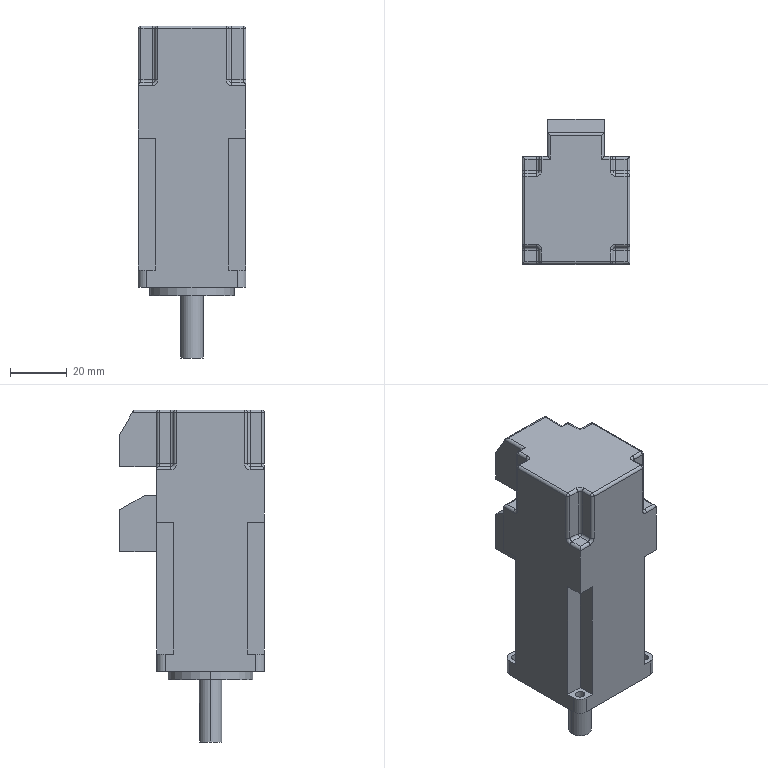Part | NX | features BREP 1 | 1 solid | 138 faces | box 38 x 51 x 117 mm | volume 133918 mm3 | cylinder 63 | plane 51 | torus 12 | sphere 12 | commonest cylinder face diameters 2 x44 3.4 x8 6 x4 8 x2 28 x2 30 x2